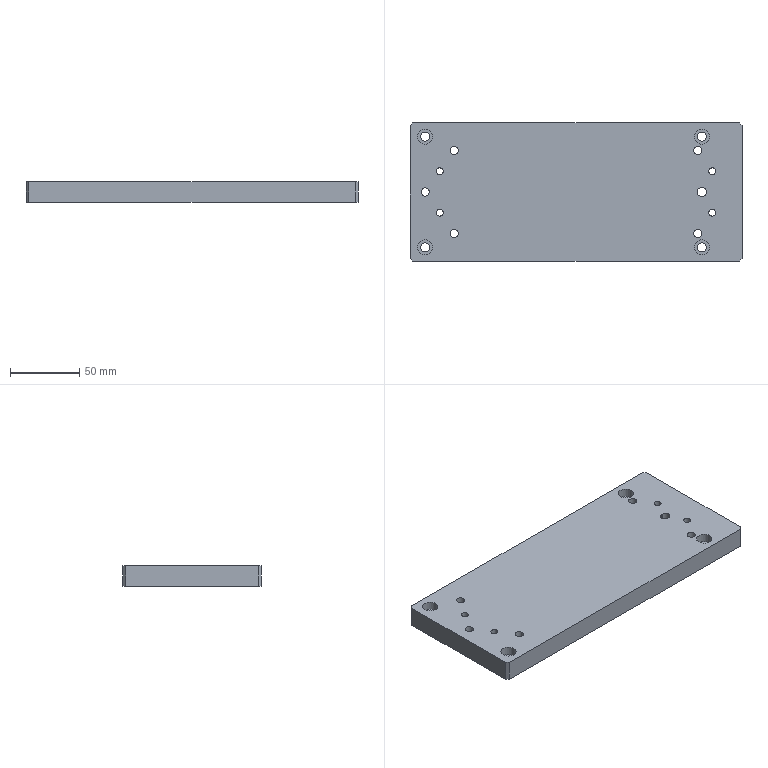Part | NX | 1 solid | 35 faces | box 240 x 100 x 15 mm | volume 352457 mm3 | cylinder 19 | plane 16 | commonest cylinder face diameters 6 x7 5 x4 6.6 x4 11 x4
STEP:
#1=CARTESIAN_POINT('',(-118.,50.,15.));
#2=VERTEX_POINT('',#1);
#3=CARTESIAN_POINT('',(-120.,48.,15.));
#4=VERTEX_POINT('',#3);
#5=CARTESIAN_POINT('',(-84.,84.,15.));
#6=DIRECTION('',(-0.7071,-0.7071,0.));
#7=VECTOR('',#6,1000.);
#8=LINE('',#5,#7);
#9=EDGE_CURVE('',#2,#4,#8,.T.);
#10=ORIENTED_EDGE('',*,*,#9,.F.);
#11=CARTESIAN_POINT('',(-118.,50.,0.));
#12=VERTEX_POINT('',#11);
#13=CARTESIAN_POINT('',(-118.,50.,15.));
#14=DIRECTION('',(0.,0.,1.));
#15=VECTOR('',#14,1000.);
#16=LINE('',#13,#15);
#17=EDGE_CURVE('',#12,#2,#16,.T.);
#18=ORIENTED_EDGE('',*,*,#17,.F.);
#19=CARTESIAN_POINT('',(-120.,48.,0.));
#20=VERTEX_POINT('',#19);
#21=CARTESIAN_POINT('',(-120.,48.,0.));
#22=DIRECTION('',(0.7071,0.7071,0.));
#23=VECTOR('',#22,1000.);
#24=LINE('',#21,#23);
#25=EDGE_CURVE('',#20,#12,#24,.T.);
#26=ORIENTED_EDGE('',*,*,#25,.F.);
#27=CARTESIAN_POINT('',(-120.,48.,15.));
#28=DIRECTION('',(0.,0.,-1.));
#29=VECTOR('',#28,1000.);
#30=LINE('',#27,#29);
#31=EDGE_CURVE('',#4,#20,#30,.T.);
#32=ORIENTED_EDGE('',*,*,#31,.F.);
#33=EDGE_LOOP('',(#10,#18,#26,#32));
#34=FACE_BOUND('',#33,.T.);
#35=CARTESIAN_POINT('',(-120.,48.,15.));
#36=DIRECTION('',(0.7071,-0.7071,0.));
#37=DIRECTION('',(0.,0.,-1.));
#38=AXIS2_PLACEMENT_3D('',#35,#36,#37);
#39=PLANE('',#38);
#40=ADVANCED_FACE('',(#34),#39,.F.);
#41=CARTESIAN_POINT('',(-120.,-48.,15.));
#42=VERTEX_POINT('',#41);
#43=CARTESIAN_POINT('',(-118.,-50.,15.));
#44=VERTEX_POINT('',#43);
#45=CARTESIAN_POINT('',(-84.,-84.,15.));
#46=DIRECTION('',(0.7071,-0.7071,0.));
#47=VECTOR('',#46,1000.);
#48=LINE('',#45,#47);
#49=EDGE_CURVE('',#42,#44,#48,.T.);
#50=ORIENTED_EDGE('',*,*,#49,.F.);
#51=CARTESIAN_POINT('',(-120.,-48.,0.));
#52=VERTEX_POINT('',#51);
#53=CARTESIAN_POINT('',(-120.,-48.,15.));
#54=DIRECTION('',(0.,0.,1.));
#55=VECTOR('',#54,1000.);
#56=LINE('',#53,#55);
#57=EDGE_CURVE('',#52,#42,#56,.T.);
#58=ORIENTED_EDGE('',*,*,#57,.F.);
#59=CARTESIAN_POINT('',(-118.,-50.,0.));
#60=VERTEX_POINT('',#59);
#61=CARTESIAN_POINT('',(-118.,-50.,0.));
#62=DIRECTION('',(-0.7071,0.7071,0.));
#63=VECTOR('',#62,1000.);
#64=LINE('',#61,#63);
#65=EDGE_CURVE('',#60,#52,#64,.T.);
#66=ORIENTED_EDGE('',*,*,#65,.F.);
#67=CARTESIAN_POINT('',(-118.,-50.,15.));
#68=DIRECTION('',(0.,0.,-1.));
#69=VECTOR('',#68,1000.);
#70=LINE('',#67,#69);
#71=EDGE_CURVE('',#44,#60,#70,.T.);
#72=ORIENTED_EDGE('',*,*,#71,.F.);
#73=EDGE_LOOP('',(#50,#58,#66,#72));
#74=FACE_BOUND('',#73,.T.);
#75=CARTESIAN_POINT('',(-118.,-50.,15.));
#76=DIRECTION('',(0.7071,0.7071,0.));
#77=DIRECTION('',(0.,0.,-1.));
#78=AXIS2_PLACEMENT_3D('',#75,#76,#77);
#79=PLANE('',#78);
#80=ADVANCED_FACE('',(#74),#79,.F.);
#81=CARTESIAN_POINT('',(118.,-50.,15.));
#82=VERTEX_POINT('',#81);
#83=CARTESIAN_POINT('',(120.,-48.,15.));
#84=VERTEX_POINT('',#83);
#85=CARTESIAN_POINT('',(84.,-84.,15.));
#86=DIRECTION('',(0.7071,0.7071,0.));
#87=VECTOR('',#86,1000.);
#88=LINE('',#85,#87);
#89=EDGE_CURVE('',#82,#84,#88,.T.);
#90=ORIENTED_EDGE('',*,*,#89,.F.);
#91=CARTESIAN_POINT('',(118.,-50.,0.));
#92=VERTEX_POINT('',#91);
#93=CARTESIAN_POINT('',(118.,-50.,15.));
#94=DIRECTION('',(0.,0.,1.));
#95=VECTOR('',#94,1000.);
#96=LINE('',#93,#95);
#97=EDGE_CURVE('',#92,#82,#96,.T.);
#98=ORIENTED_EDGE('',*,*,#97,.F.);
#99=CARTESIAN_POINT('',(120.,-48.,0.));
#100=VERTEX_POINT('',#99);
#101=CARTESIAN_POINT('',(120.,-48.,0.));
#102=DIRECTION('',(-0.7071,-0.7071,0.));
#103=VECTOR('',#102,1000.);
#104=LINE('',#101,#103);
#105=EDGE_CURVE('',#100,#92,#104,.T.);
#106=ORIENTED_EDGE('',*,*,#105,.F.);
#107=CARTESIAN_POINT('',(120.,-48.,15.));
#108=DIRECTION('',(0.,0.,-1.));
#109=VECTOR('',#108,1000.);
#110=LINE('',#107,#109);
#111=EDGE_CURVE('',#84,#100,#110,.T.);
#112=ORIENTED_EDGE('',*,*,#111,.F.);
#113=EDGE_LOOP('',(#90,#98,#106,#112));
#114=FACE_BOUND('',#113,.T.);
#115=CARTESIAN_POINT('',(120.,-48.,15.));
#116=DIRECTION('',(-0.7071,0.7071,0.));
#117=DIRECTION('',(0.,0.,-1.));
#118=AXIS2_PLACEMENT_3D('',#115,#116,#117);
#119=PLANE('',#118);
#120=ADVANCED_FACE('',(#114),#119,.F.);
#121=CARTESIAN_POINT('',(120.,48.,15.));
#122=VERTEX_POINT('',#121);
#123=CARTESIAN_POINT('',(118.,50.,15.));
#124=VERTEX_POINT('',#123);
#125=CARTESIAN_POINT('',(84.,84.,15.));
#126=DIRECTION('',(-0.7071,0.7071,0.));
#127=VECTOR('',#126,1000.);
#128=LINE('',#125,#127);
#129=EDGE_CURVE('',#122,#124,#128,.T.);
#130=ORIENTED_EDGE('',*,*,#129,.F.);
#131=CARTESIAN_POINT('',(120.,48.,0.));
#132=VERTEX_POINT('',#131);
#133=CARTESIAN_POINT('',(120.,48.,15.));
#134=DIRECTION('',(0.,0.,1.));
#135=VECTOR('',#134,1000.);
#136=LINE('',#133,#135);
#137=EDGE_CURVE('',#132,#122,#136,.T.);
#138=ORIENTED_EDGE('',*,*,#137,.F.);
#139=CARTESIAN_POINT('',(118.,50.,0.));
#140=VERTEX_POINT('',#139);
#141=CARTESIAN_POINT('',(118.,50.,0.));
#142=DIRECTION('',(0.7071,-0.7071,0.));
#143=VECTOR('',#142,1000.);
#144=LINE('',#141,#143);
#145=EDGE_CURVE('',#140,#132,#144,.T.);
#146=ORIENTED_EDGE('',*,*,#145,.F.);
#147=CARTESIAN_POINT('',(118.,50.,15.));
#148=DIRECTION('',(0.,0.,-1.));
#149=VECTOR('',#148,1000.);
#150=LINE('',#147,#149);
#151=EDGE_CURVE('',#124,#140,#150,.T.);
#152=ORIENTED_EDGE('',*,*,#151,.F.);
#153=EDGE_LOOP('',(#130,#138,#146,#152));
#154=FACE_BOUND('',#153,.T.);
#155=CARTESIAN_POINT('',(118.,50.,15.));
#156=DIRECTION('',(-0.7071,-0.7071,0.));
#157=DIRECTION('',(0.,0.,-1.));
#158=AXIS2_PLACEMENT_3D('',#155,#156,#157);
#159=PLANE('',#158);
#160=ADVANCED_FACE('',(#154),#159,.F.);
#161=CARTESIAN_POINT('',(91.5,-3.,15.));
#162=VERTEX_POINT('',#161);
#163=CARTESIAN_POINT('',(91.5,-3.,0.));
#164=VERTEX_POINT('',#163);
#165=CARTESIAN_POINT('',(91.5,-3.,15.));
#166=DIRECTION('',(0.,0.,-1.));
#167=VECTOR('',#166,1000.);
#168=LINE('',#165,#167);
#169=EDGE_CURVE('',#162,#164,#168,.T.);
#170=ORIENTED_EDGE('',*,*,#169,.T.);
#171=CARTESIAN_POINT('',(90.5,-3.,0.));
#172=VERTEX_POINT('',#171);
#173=CARTESIAN_POINT('',(90.5,-3.,0.));
#174=DIRECTION('',(1.,0.,0.));
#175=VECTOR('',#174,1000.);
#176=LINE('',#173,#175);
#177=EDGE_CURVE('',#172,#164,#176,.T.);
#178=ORIENTED_EDGE('',*,*,#177,.F.);
#179=CARTESIAN_POINT('',(90.5,-3.,15.));
#180=VERTEX_POINT('',#179);
#181=CARTESIAN_POINT('',(90.5,-3.,15.));
#182=DIRECTION('',(0.,0.,1.));
#183=VECTOR('',#182,1000.);
#184=LINE('',#181,#183);
#185=EDGE_CURVE('',#172,#180,#184,.T.);
#186=ORIENTED_EDGE('',*,*,#185,.T.);
#187=CARTESIAN_POINT('',(90.5,-3.,15.));
#188=DIRECTION('',(1.,0.,0.));
#189=VECTOR('',#188,1000.);
#190=LINE('',#187,#189);
#191=EDGE_CURVE('',#180,#162,#190,.T.);
#192=ORIENTED_EDGE('',*,*,#191,.T.);
#193=EDGE_LOOP('',(#170,#178,#186,#192));
#194=FACE_BOUND('',#193,.T.);
#195=CARTESIAN_POINT('',(90.5,-3.,15.));
#196=DIRECTION('',(0.,-1.,0.));
#197=DIRECTION('',(1.,0.,0.));
#198=AXIS2_PLACEMENT_3D('',#195,#196,#197);
#199=PLANE('',#198);
#200=ADVANCED_FACE('',(#194),#199,.F.);
#201=CARTESIAN_POINT('',(91.5,3.,0.));
#202=VERTEX_POINT('',#201);
#203=CARTESIAN_POINT('',(91.5,3.,15.));
#204=VERTEX_POINT('',#203);
#205=CARTESIAN_POINT('',(91.5,3.,15.));
#206=DIRECTION('',(0.,0.,1.));
#207=VECTOR('',#206,1000.);
#208=LINE('',#205,#207);
#209=EDGE_CURVE('',#202,#204,#208,.T.);
#210=ORIENTED_EDGE('',*,*,#209,.T.);
#211=CARTESIAN_POINT('',(90.5,3.,15.));
#212=VERTEX_POINT('',#211);
#213=CARTESIAN_POINT('',(90.5,3.,15.));
#214=DIRECTION('',(1.,0.,0.));
#215=VECTOR('',#214,1000.);
#216=LINE('',#213,#215);
#217=EDGE_CURVE('',#212,#204,#216,.T.);
#218=ORIENTED_EDGE('',*,*,#217,.F.);
#219=CARTESIAN_POINT('',(90.5,3.,0.));
#220=VERTEX_POINT('',#219);
#221=CARTESIAN_POINT('',(90.5,3.,15.));
#222=DIRECTION('',(0.,0.,-1.));
#223=VECTOR('',#222,1000.);
#224=LINE('',#221,#223);
#225=EDGE_CURVE('',#212,#220,#224,.T.);
#226=ORIENTED_EDGE('',*,*,#225,.T.);
#227=CARTESIAN_POINT('',(90.5,3.,0.));
#228=DIRECTION('',(1.,0.,0.));
#229=VECTOR('',#228,1000.);
#230=LINE('',#227,#229);
#231=EDGE_CURVE('',#220,#202,#230,.T.);
#232=ORIENTED_EDGE('',*,*,#231,.T.);
#233=EDGE_LOOP('',(#210,#218,#226,#232));
#234=FACE_BOUND('',#233,.T.);
#235=CARTESIAN_POINT('',(90.5,3.,15.));
#236=DIRECTION('',(0.,1.,0.));
#237=DIRECTION('',(-1.,0.,0.));
#238=AXIS2_PLACEMENT_3D('',#235,#236,#237);
#239=PLANE('',#238);
#240=ADVANCED_FACE('',(#234),#239,.F.);
#241=CARTESIAN_POINT('',(90.5,0.,15.));
#242=DIRECTION('',(0.,0.,1.));
#243=DIRECTION('',(1.,0.,0.));
#244=AXIS2_PLACEMENT_3D('',#241,#242,#243);
#245=CIRCLE('',#244,3.);
#246=EDGE_CURVE('',#212,#180,#245,.T.);
#247=ORIENTED_EDGE('',*,*,#246,.T.);
#248=ORIENTED_EDGE('',*,*,#185,.F.);
#249=CARTESIAN_POINT('',(90.5,0.,0.));
#250=DIRECTION('',(0.,0.,1.));
#251=DIRECTION('',(1.,0.,0.));
#252=AXIS2_PLACEMENT_3D('',#249,#250,#251);
#253=CIRCLE('',#252,3.);
#254=EDGE_CURVE('',#220,#172,#253,.T.);
#255=ORIENTED_EDGE('',*,*,#254,.F.);
#256=ORIENTED_EDGE('',*,*,#225,.F.);
#257=EDGE_LOOP('',(#247,#248,#255,#256));
#258=FACE_BOUND('',#257,.T.);
#259=CARTESIAN_POINT('',(90.5,0.,15.));
#260=DIRECTION('',(0.,0.,1.));
#261=DIRECTION('',(1.,0.,0.));
#262=AXIS2_PLACEMENT_3D('',#259,#260,#261);
#263=CYLINDRICAL_SURFACE('',#262,3.);
#264=ADVANCED_FACE('',(#258),#263,.F.);
#265=CARTESIAN_POINT('',(-103.5,-40.,8.6));
#266=VERTEX_POINT('',#265);
#267=CARTESIAN_POINT('',(-109.,-40.,8.6));
#268=DIRECTION('',(0.,0.,1.));
#269=DIRECTION('',(1.,0.,0.));
#270=AXIS2_PLACEMENT_3D('',#267,#268,#269);
#271=CIRCLE('',#270,5.5);
#272=EDGE_CURVE('',#266,#266,#271,.T.);
#273=ORIENTED_EDGE('',*,*,#272,.T.);
#274=EDGE_LOOP('',(#273));
#275=FACE_BOUND('',#274,.T.);
#276=CARTESIAN_POINT('',(-105.7,-40.,8.6));
#277=VERTEX_POINT('',#276);
#278=CARTESIAN_POINT('',(-109.,-40.,8.6));
#279=DIRECTION('',(0.,0.,1.));
#280=DIRECTION('',(1.,0.,0.));
#281=AXIS2_PLACEMENT_3D('',#278,#279,#280);
#282=CIRCLE('',#281,3.3);
#283=EDGE_CURVE('',#277,#277,#282,.T.);
#284=ORIENTED_EDGE('',*,*,#283,.F.);
#285=EDGE_LOOP('',(#284));
#286=FACE_BOUND('',#285,.T.);
#287=CARTESIAN_POINT('',(-105.7,-40.,8.6));
#288=DIRECTION('',(0.,0.,-1.));
#289=DIRECTION('',(-1.,0.,0.));
#290=AXIS2_PLACEMENT_3D('',#287,#288,#289);
#291=PLANE('',#290);
#292=ADVANCED_FACE('',(#275,#286),#291,.F.);
#293=CARTESIAN_POINT('',(-114.5,40.,8.6));
#294=VERTEX_POINT('',#293);
#295=CARTESIAN_POINT('',(-109.,40.,8.6));
#296=DIRECTION('',(0.,0.,1.));
#297=DIRECTION('',(-1.,0.,0.));
#298=AXIS2_PLACEMENT_3D('',#295,#296,#297);
#299=CIRCLE('',#298,5.5);
#300=EDGE_CURVE('',#294,#294,#299,.T.);
#301=ORIENTED_EDGE('',*,*,#300,.T.);
#302=EDGE_LOOP('',(#301));
#303=FACE_BOUND('',#302,.T.);
#304=CARTESIAN_POINT('',(-112.3,40.,8.6));
#305=VERTEX_POINT('',#304);
#306=CARTESIAN_POINT('',(-109.,40.,8.6));
#307=DIRECTION('',(0.,0.,1.));
#308=DIRECTION('',(-1.,0.,0.));
#309=AXIS2_PLACEMENT_3D('',#306,#307,#308);
#310=CIRCLE('',#309,3.3);
#311=EDGE_CURVE('',#305,#305,#310,.T.);
#312=ORIENTED_EDGE('',*,*,#311,.F.);
#313=EDGE_LOOP('',(#312));
#314=FACE_BOUND('',#313,.T.);
#315=CARTESIAN_POINT('',(-105.7,-40.,8.6));
#316=DIRECTION('',(0.,0.,-1.));
#317=DIRECTION('',(-1.,0.,0.));
#318=AXIS2_PLACEMENT_3D('',#315,#316,#317);
#319=PLANE('',#318);
#320=ADVANCED_FACE('',(#303,#314),#319,.F.);
#321=CARTESIAN_POINT('',(85.5,-40.,8.6));
#322=VERTEX_POINT('',#321);
#323=CARTESIAN_POINT('',(91.,-40.,8.6));
#324=DIRECTION('',(0.,0.,1.));
#325=DIRECTION('',(-1.,0.,0.));
#326=AXIS2_PLACEMENT_3D('',#323,#324,#325);
#327=CIRCLE('',#326,5.5);
#328=EDGE_CURVE('',#322,#322,#327,.T.);
#329=ORIENTED_EDGE('',*,*,#328,.T.);
#330=EDGE_LOOP('',(#329));
#331=FACE_BOUND('',#330,.T.);
#332=CARTESIAN_POINT('',(87.7,-40.,8.6));
#333=VERTEX_POINT('',#332);
#334=CARTESIAN_POINT('',(91.,-40.,8.6));
#335=DIRECTION('',(0.,0.,1.));
#336=DIRECTION('',(-1.,0.,0.));
#337=AXIS2_PLACEMENT_3D('',#334,#335,#336);
#338=CIRCLE('',#337,3.3);
#339=EDGE_CURVE('',#333,#333,#338,.T.);
#340=ORIENTED_EDGE('',*,*,#339,.F.);
#341=EDGE_LOOP('',(#340));
#342=FACE_BOUND('',#341,.T.);
#343=CARTESIAN_POINT('',(-105.7,-40.,8.6));
#344=DIRECTION('',(0.,0.,-1.));
#345=DIRECTION('',(-1.,0.,0.));
#346=AXIS2_PLACEMENT_3D('',#343,#344,#345);
#347=PLANE('',#346);
#348=ADVANCED_FACE('',(#331,#342),#347,.F.);
#349=CARTESIAN_POINT('',(85.5,40.,8.6));
#350=VERTEX_POINT('',#349);
#351=CARTESIAN_POINT('',(91.,40.,8.6));
#352=DIRECTION('',(0.,0.,1.));
#353=DIRECTION('',(-1.,0.,0.));
#354=AXIS2_PLACEMENT_3D('',#351,#352,#353);
#355=CIRCLE('',#354,5.5);
#356=EDGE_CURVE('',#350,#350,#355,.T.);
#357=ORIENTED_EDGE('',*,*,#356,.T.);
#358=EDGE_LOOP('',(#357));
#359=FACE_BOUND('',#358,.T.);
#360=CARTESIAN_POINT('',(87.7,40.,8.6));
#361=VERTEX_POINT('',#360);
#362=CARTESIAN_POINT('',(91.,40.,8.6));
#363=DIRECTION('',(0.,0.,1.));
#364=DIRECTION('',(-1.,0.,0.));
#365=AXIS2_PLACEMENT_3D('',#362,#363,#364);
#366=CIRCLE('',#365,3.3);
#367=EDGE_CURVE('',#361,#361,#366,.T.);
#368=ORIENTED_EDGE('',*,*,#367,.F.);
#369=EDGE_LOOP('',(#368));
#370=FACE_BOUND('',#369,.T.);
#371=CARTESIAN_POINT('',(-105.7,-40.,8.6));
#372=DIRECTION('',(0.,0.,-1.));
#373=DIRECTION('',(-1.,0.,0.));
#374=AXIS2_PLACEMENT_3D('',#371,#372,#373);
#375=PLANE('',#374);
#376=ADVANCED_FACE('',(#359,#370),#375,.F.);
#377=CARTESIAN_POINT('',(-120.,50.,0.));
#378=DIRECTION('',(-1.,0.,0.));
#379=VECTOR('',#378,1000.);
#380=LINE('',#377,#379);
#381=EDGE_CURVE('',#140,#12,#380,.T.);
#382=ORIENTED_EDGE('',*,*,#381,.F.);
#383=ORIENTED_EDGE('',*,*,#145,.T.);
#384=CARTESIAN_POINT('',(120.,50.,0.));
#385=DIRECTION('',(0.,1.,0.));
#386=VECTOR('',#385,1000.);
#387=LINE('',#384,#386);
#388=EDGE_CURVE('',#100,#132,#387,.T.);
#389=ORIENTED_EDGE('',*,*,#388,.F.);
#390=ORIENTED_EDGE('',*,*,#105,.T.);
#391=CARTESIAN_POINT('',(-120.,-50.,0.));
#392=DIRECTION('',(1.,0.,0.));
#393=VECTOR('',#392,1000.);
#394=LINE('',#391,#393);
#395=EDGE_CURVE('',#60,#92,#394,.T.);
#396=ORIENTED_EDGE('',*,*,#395,.F.);
#397=ORIENTED_EDGE('',*,*,#65,.T.);
#398=CARTESIAN_POINT('',(-120.,50.,0.));
#399=DIRECTION('',(0.,-1.,0.));
#400=VECTOR('',#399,1000.);
#401=LINE('',#398,#400);
#402=EDGE_CURVE('',#20,#52,#401,.T.);
#403=ORIENTED_EDGE('',*,*,#402,.F.);
#404=ORIENTED_EDGE('',*,*,#25,.T.);
#405=EDGE_LOOP('',(#382,#383,#389,#390,#396,#397,#403,#404));
#406=FACE_BOUND('',#405,.T.);
#407=CARTESIAN_POINT('',(101.,15.,0.));
#408=VERTEX_POINT('',#407);
#409=CARTESIAN_POINT('',(98.5,15.,0.));
#410=DIRECTION('',(0.,0.,1.));
#411=DIRECTION('',(1.,0.,0.));
#412=AXIS2_PLACEMENT_3D('',#409,#410,#411);
#413=CIRCLE('',#412,2.5);
#414=EDGE_CURVE('',#408,#408,#413,.T.);
#415=ORIENTED_EDGE('',*,*,#414,.T.);
#416=EDGE_LOOP('',(#415));
#417=FACE_BOUND('',#416,.T.);
#418=CARTESIAN_POINT('',(101.,-15.,0.));
#419=VERTEX_POINT('',#418);
#420=CARTESIAN_POINT('',(98.5,-15.,0.));
#421=DIRECTION('',(0.,0.,1.));
#422=DIRECTION('',(1.,0.,0.));
#423=AXIS2_PLACEMENT_3D('',#420,#421,#422);
#424=CIRCLE('',#423,2.5);
#425=EDGE_CURVE('',#419,#419,#424,.T.);
#426=ORIENTED_EDGE('',*,*,#425,.T.);
#427=EDGE_LOOP('',(#426));
#428=FACE_BOUND('',#427,.T.);
#429=CARTESIAN_POINT('',(-96.,-15.,0.));
#430=VERTEX_POINT('',#429);
#431=CARTESIAN_POINT('',(-98.5,-15.,0.));
#432=DIRECTION('',(0.,0.,1.));
#433=DIRECTION('',(1.,0.,0.));
#434=AXIS2_PLACEMENT_3D('',#431,#432,#433);
#435=CIRCLE('',#434,2.5);
#436=EDGE_CURVE('',#430,#430,#435,.T.);
#437=ORIENTED_EDGE('',*,*,#436,.T.);
#438=EDGE_LOOP('',(#437));
#439=FACE_BOUND('',#438,.T.);
#440=CARTESIAN_POINT('',(-96.,15.,0.));
#441=VERTEX_POINT('',#440);
#442=CARTESIAN_POINT('',(-98.5,15.,0.));
#443=DIRECTION('',(0.,0.,1.));
#444=DIRECTION('',(1.,0.,0.));
#445=AXIS2_PLACEMENT_3D('',#442,#443,#444);
#446=CIRCLE('',#445,2.5);
#447=EDGE_CURVE('',#441,#441,#446,.T.);
#448=ORIENTED_EDGE('',*,*,#447,.T.);
#449=EDGE_LOOP('',(#448));
#450=FACE_BOUND('',#449,.T.);
#451=CARTESIAN_POINT('',(94.3,40.,0.));
#452=VERTEX_POINT('',#451);
#453=CARTESIAN_POINT('',(91.,40.,0.));
#454=DIRECTION('',(0.,0.,1.));
#455=DIRECTION('',(1.,0.,0.));
#456=AXIS2_PLACEMENT_3D('',#453,#454,#455);
#457=CIRCLE('',#456,3.3);
#458=EDGE_CURVE('',#452,#452,#457,.T.);
#459=ORIENTED_EDGE('',*,*,#458,.T.);
#460=EDGE_LOOP('',(#459));
#461=FACE_BOUND('',#460,.T.);
#462=CARTESIAN_POINT('',(94.3,-40.,0.));
#463=VERTEX_POINT('',#462);
#464=CARTESIAN_POINT('',(91.,-40.,0.));
#465=DIRECTION('',(0.,0.,1.));
#466=DIRECTION('',(1.,0.,0.));
#467=AXIS2_PLACEMENT_3D('',#464,#465,#466);
#468=CIRCLE('',#467,3.3);
#469=EDGE_CURVE('',#463,#463,#468,.T.);
#470=ORIENTED_EDGE('',*,*,#469,.T.);
#471=EDGE_LOOP('',(#470));
#472=FACE_BOUND('',#471,.T.);
#473=CARTESIAN_POINT('',(-105.7,40.,0.));
#474=VERTEX_POINT('',#473);
#475=CARTESIAN_POINT('',(-109.,40.,0.));
#476=DIRECTION('',(0.,0.,1.));
#477=DIRECTION('',(1.,0.,0.));
#478=AXIS2_PLACEMENT_3D('',#475,#476,#477);
#479=CIRCLE('',#478,3.3);
#480=EDGE_CURVE('',#474,#474,#479,.T.);
#481=ORIENTED_EDGE('',*,*,#480,.T.);
#482=EDGE_LOOP('',(#481));
#483=FACE_BOUND('',#482,.T.);
#484=CARTESIAN_POINT('',(-105.7,-40.,0.));
#485=VERTEX_POINT('',#484);
#486=CARTESIAN_POINT('',(-109.,-40.,0.));
#487=DIRECTION('',(0.,0.,1.));
#488=DIRECTION('',(1.,0.,0.));
#489=AXIS2_PLACEMENT_3D('',#486,#487,#488);
#490=CIRCLE('',#489,3.3);
#491=EDGE_CURVE('',#485,#485,#490,.T.);
#492=ORIENTED_EDGE('',*,*,#491,.T.);
#493=EDGE_LOOP('',(#492));
#494=FACE_BOUND('',#493,.T.);
#495=CARTESIAN_POINT('',(-106.,0.,0.));
#496=VERTEX_POINT('',#495);
#497=CARTESIAN_POINT('',(-109.,0.,0.));
#498=DIRECTION('',(0.,0.,1.));
#499=DIRECTION('',(1.,0.,0.));
#500=AXIS2_PLACEMENT_3D('',#497,#498,#499);
#501=CIRCLE('',#500,3.);
#502=EDGE_CURVE('',#496,#496,#501,.T.);
#503=ORIENTED_EDGE('',*,*,#502,.T.);
#504=EDGE_LOOP('',(#503));
#505=FACE_BOUND('',#504,.T.);
#506=ORIENTED_EDGE('',*,*,#177,.T.);
#507=CARTESIAN_POINT('',(91.5,0.,0.));
#508=DIRECTION('',(0.,0.,1.));
#509=DIRECTION('',(1.,0.,0.));
#510=AXIS2_PLACEMENT_3D('',#507,#508,#509);
#511=CIRCLE('',#510,3.);
#512=EDGE_CURVE('',#164,#202,#511,.T.);
#513=ORIENTED_EDGE('',*,*,#512,.T.);
#514=ORIENTED_EDGE('',*,*,#231,.F.);
#515=ORIENTED_EDGE('',*,*,#254,.T.);
#516=EDGE_LOOP('',(#506,#513,#514,#515));
#517=FACE_BOUND('',#516,.T.);
#518=CARTESIAN_POINT('',(91.,-30.,0.));
#519=VERTEX_POINT('',#518);
#520=CARTESIAN_POINT('',(88.,-30.,0.));
#521=DIRECTION('',(0.,0.,1.));
#522=DIRECTION('',(1.,0.,0.));
#523=AXIS2_PLACEMENT_3D('',#520,#521,#522);
#524=CIRCLE('',#523,3.);
#525=EDGE_CURVE('',#519,#519,#524,.T.);
#526=ORIENTED_EDGE('',*,*,#525,.T.);
#527=EDGE_LOOP('',(#526));
#528=FACE_BOUND('',#527,.T.);
#529=CARTESIAN_POINT('',(91.,30.,0.));
#530=VERTEX_POINT('',#529);
#531=CARTESIAN_POINT('',(88.,30.,0.));
#532=DIRECTION('',(0.,0.,1.));
#533=DIRECTION('',(1.,0.,0.));
#534=AXIS2_PLACEMENT_3D('',#531,#532,#533);
#535=CIRCLE('',#534,3.);
#536=EDGE_CURVE('',#530,#530,#535,.T.);
#537=ORIENTED_EDGE('',*,*,#536,.T.);
#538=EDGE_LOOP('',(#537));
#539=FACE_BOUND('',#538,.T.);
#540=CARTESIAN_POINT('',(-85.,-30.,0.));
#541=VERTEX_POINT('',#540);
#542=CARTESIAN_POINT('',(-88.,-30.,0.));
#543=DIRECTION('',(0.,0.,1.));
#544=DIRECTION('',(1.,0.,0.));
#545=AXIS2_PLACEMENT_3D('',#542,#543,#544);
#546=CIRCLE('',#545,3.);
#547=EDGE_CURVE('',#541,#541,#546,.T.);
#548=ORIENTED_EDGE('',*,*,#547,.T.);
#549=EDGE_LOOP('',(#548));
#550=FACE_BOUND('',#549,.T.);
#551=CARTESIAN_POINT('',(-85.,30.,0.));
#552=VERTEX_POINT('',#551);
#553=CARTESIAN_POINT('',(-88.,30.,0.));
#554=DIRECTION('',(0.,0.,1.));
#555=DIRECTION('',(1.,0.,0.));
#556=AXIS2_PLACEMENT_3D('',#553,#554,#555);
#557=CIRCLE('',#556,3.);
#558=EDGE_CURVE('',#552,#552,#557,.T.);
#559=ORIENTED_EDGE('',*,*,#558,.T.);
#560=EDGE_LOOP('',(#559));
#561=FACE_BOUND('',#560,.T.);
#562=CARTESIAN_POINT('',(0.,0.,0.));
#563=DIRECTION('',(0.,0.,1.));
#564=DIRECTION('',(1.,0.,0.));
#565=AXIS2_PLACEMENT_3D('',#562,#563,#564);
#566=PLANE('',#565);
#567=ADVANCED_FACE('',(#406,#417,#428,#439,#450,#461,#472,#483,#494,#505,#517,#528,#539,#550,#561),#566,.F.);
#568=ORIENTED_EDGE('',*,*,#395,.T.);
#569=ORIENTED_EDGE('',*,*,#97,.T.);
#570=CARTESIAN_POINT('',(-120.,-50.,15.));
#571=DIRECTION('',(1.,0.,0.));
#572=VECTOR('',#571,1000.);
#573=LINE('',#570,#572);
#574=EDGE_CURVE('',#44,#82,#573,.T.);
#575=ORIENTED_EDGE('',*,*,#574,.F.);
#576=ORIENTED_EDGE('',*,*,#71,.T.);
#577=EDGE_LOOP('',(#568,#569,#575,#576));
#578=FACE_BOUND('',#577,.T.);
#579=CARTESIAN_POINT('',(-120.,-50.,15.));
#580=DIRECTION('',(0.,1.,0.));
#581=DIRECTION('',(0.,0.,1.));
#582=AXIS2_PLACEMENT_3D('',#579,#580,#581);
#583=PLANE('',#582);
#584=ADVANCED_FACE('',(#578),#583,.F.);
#585=ORIENTED_EDGE('',*,*,#402,.T.);
#586=ORIENTED_EDGE('',*,*,#57,.T.);
#587=CARTESIAN_POINT('',(-120.,50.,15.));
#588=DIRECTION('',(0.,-1.,0.));
#589=VECTOR('',#588,1000.);
#590=LINE('',#587,#589);
#591=EDGE_CURVE('',#4,#42,#590,.T.);
#592=ORIENTED_EDGE('',*,*,#591,.F.);
#593=ORIENTED_EDGE('',*,*,#31,.T.);
#594=EDGE_LOOP('',(#585,#586,#592,#593));
#595=FACE_BOUND('',#594,.T.);
#596=CARTESIAN_POINT('',(-120.,50.,15.));
#597=DIRECTION('',(1.,0.,0.));
#598=DIRECTION('',(0.,1.,0.));
#599=AXIS2_PLACEMENT_3D('',#596,#597,#598);
#600=PLANE('',#599);
#601=ADVANCED_FACE('',(#595),#600,.F.);
#602=CARTESIAN_POINT('',(-120.,50.,15.));
#603=DIRECTION('',(-1.,0.,0.));
#604=VECTOR('',#603,1000.);
#605=LINE('',#602,#604);
#606=EDGE_CURVE('',#124,#2,#605,.T.);
#607=ORIENTED_EDGE('',*,*,#606,.F.);
#608=ORIENTED_EDGE('',*,*,#151,.T.);
#609=ORIENTED_EDGE('',*,*,#381,.T.);
#610=ORIENTED_EDGE('',*,*,#17,.T.);
#611=EDGE_LOOP('',(#607,#608,#609,#610));
#612=FACE_BOUND('',#611,.T.);
#613=CARTESIAN_POINT('',(-120.,50.,15.));
#614=DIRECTION('',(0.,-1.,0.));
#615=DIRECTION('',(0.,0.,-1.));
#616=AXIS2_PLACEMENT_3D('',#613,#614,#615);
#617=PLANE('',#616);
#618=ADVANCED_FACE('',(#612),#617,.F.);
#619=ORIENTED_EDGE('',*,*,#388,.T.);
#620=ORIENTED_EDGE('',*,*,#137,.T.);
#621=CARTESIAN_POINT('',(120.,50.,15.));
#622=DIRECTION('',(0.,1.,0.));
#623=VECTOR('',#622,1000.);
#624=LINE('',#621,#623);
#625=EDGE_CURVE('',#84,#122,#624,.T.);
#626=ORIENTED_EDGE('',*,*,#625,.F.);
#627=ORIENTED_EDGE('',*,*,#111,.T.);
#628=EDGE_LOOP('',(#619,#620,#626,#627));
#629=FACE_BOUND('',#628,.T.);
#630=CARTESIAN_POINT('',(120.,50.,15.));
#631=DIRECTION('',(-1.,0.,0.));
#632=DIRECTION('',(0.,0.,1.));
#633=AXIS2_PLACEMENT_3D('',#630,#631,#632);
#634=PLANE('',#633);
#635=ADVANCED_FACE('',(#629),#634,.F.);
#636=ORIENTED_EDGE('',*,*,#246,.F.);
#637=ORIENTED_EDGE('',*,*,#217,.T.);
#638=CARTESIAN_POINT('',(91.5,0.,15.));
#639=DIRECTION('',(0.,0.,1.));
#640=DIRECTION('',(1.,0.,0.));
#641=AXIS2_PLACEMENT_3D('',#638,#639,#640);
#642=CIRCLE('',#641,3.);
#643=EDGE_CURVE('',#162,#204,#642,.T.);
#644=ORIENTED_EDGE('',*,*,#643,.F.);
#645=ORIENTED_EDGE('',*,*,#191,.F.);
#646=EDGE_LOOP('',(#636,#637,#644,#645));
#647=FACE_BOUND('',#646,.T.);
#648=ORIENTED_EDGE('',*,*,#625,.T.);
#649=ORIENTED_EDGE('',*,*,#129,.T.);
#650=ORIENTED_EDGE('',*,*,#606,.T.);
#651=ORIENTED_EDGE('',*,*,#9,.T.);
#652=ORIENTED_EDGE('',*,*,#591,.T.);
#653=ORIENTED_EDGE('',*,*,#49,.T.);
#654=ORIENTED_EDGE('',*,*,#574,.T.);
#655=ORIENTED_EDGE('',*,*,#89,.T.);
#656=EDGE_LOOP('',(#648,#649,#650,#651,#652,#653,#654,#655));
#657=FACE_BOUND('',#656,.T.);
#658=CARTESIAN_POINT('',(101.,15.,15.));
#659=VERTEX_POINT('',#658);
#660=CARTESIAN_POINT('',(98.5,15.,15.));
#661=DIRECTION('',(0.,0.,1.));
#662=DIRECTION('',(1.,0.,0.));
#663=AXIS2_PLACEMENT_3D('',#660,#661,#662);
#664=CIRCLE('',#663,2.5);
#665=EDGE_CURVE('',#659,#659,#664,.T.);
#666=ORIENTED_EDGE('',*,*,#665,.F.);
#667=EDGE_LOOP('',(#666));
#668=FACE_BOUND('',#667,.T.);
#669=CARTESIAN_POINT('',(101.,-15.,15.));
#670=VERTEX_POINT('',#669);
#671=CARTESIAN_POINT('',(98.5,-15.,15.));
#672=DIRECTION('',(0.,0.,1.));
#673=DIRECTION('',(1.,0.,0.));
#674=AXIS2_PLACEMENT_3D('',#671,#672,#673);
#675=CIRCLE('',#674,2.5);
#676=EDGE_CURVE('',#670,#670,#675,.T.);
#677=ORIENTED_EDGE('',*,*,#676,.F.);
#678=EDGE_LOOP('',(#677));
#679=FACE_BOUND('',#678,.T.);
#680=CARTESIAN_POINT('',(-96.,-15.,15.));
#681=VERTEX_POINT('',#680);
#682=CARTESIAN_POINT('',(-98.5,-15.,15.));
#683=DIRECTION('',(0.,0.,1.));
#684=DIRECTION('',(1.,0.,0.));
#685=AXIS2_PLACEMENT_3D('',#682,#683,#684);
#686=CIRCLE('',#685,2.5);
#687=EDGE_CURVE('',#681,#681,#686,.T.);
#688=ORIENTED_EDGE('',*,*,#687,.F.);
#689=EDGE_LOOP('',(#688));
#690=FACE_BOUND('',#689,.T.);
#691=CARTESIAN_POINT('',(-96.,15.,15.));
#692=VERTEX_POINT('',#691);
#693=CARTESIAN_POINT('',(-98.5,15.,15.));
#694=DIRECTION('',(0.,0.,1.));
#695=DIRECTION('',(1.,0.,0.));
#696=AXIS2_PLACEMENT_3D('',#693,#694,#695);
#697=CIRCLE('',#696,2.5);
#698=EDGE_CURVE('',#692,#692,#697,.T.);
#699=ORIENTED_EDGE('',*,*,#698,.F.);
#700=EDGE_LOOP('',(#699));
#701=FACE_BOUND('',#700,.T.);
#702=CARTESIAN_POINT('',(96.5,40.,15.));
#703=VERTEX_POINT('',#702);
#704=CARTESIAN_POINT('',(91.,40.,15.));
#705=DIRECTION('',(0.,0.,1.));
#706=DIRECTION('',(1.,0.,0.));
#707=AXIS2_PLACEMENT_3D('',#704,#705,#706);
#708=CIRCLE('',#707,5.5);
#709=EDGE_CURVE('',#703,#703,#708,.T.);
#710=ORIENTED_EDGE('',*,*,#709,.F.);
#711=EDGE_LOOP('',(#710));
#712=FACE_BOUND('',#711,.T.);
#713=CARTESIAN_POINT('',(96.5,-40.,15.));
#714=VERTEX_POINT('',#713);
#715=CARTESIAN_POINT('',(91.,-40.,15.));
#716=DIRECTION('',(0.,0.,1.));
#717=DIRECTION('',(1.,0.,0.));
#718=AXIS2_PLACEMENT_3D('',#715,#716,#717);
#719=CIRCLE('',#718,5.5);
#720=EDGE_CURVE('',#714,#714,#719,.T.);
#721=ORIENTED_EDGE('',*,*,#720,.F.);
#722=EDGE_LOOP('',(#721));
#723=FACE_BOUND('',#722,.T.);
#724=CARTESIAN_POINT('',(-103.5,40.,15.));
#725=VERTEX_POINT('',#724);
#726=CARTESIAN_POINT('',(-109.,40.,15.));
#727=DIRECTION('',(0.,0.,1.));
#728=DIRECTION('',(1.,0.,0.));
#729=AXIS2_PLACEMENT_3D('',#726,#727,#728);
#730=CIRCLE('',#729,5.5);
#731=EDGE_CURVE('',#725,#725,#730,.T.);
#732=ORIENTED_EDGE('',*,*,#731,.F.);
#733=EDGE_LOOP('',(#732));
#734=FACE_BOUND('',#733,.T.);
#735=CARTESIAN_POINT('',(-103.5,-40.,15.));
#736=VERTEX_POINT('',#735);
#737=CARTESIAN_POINT('',(-109.,-40.,15.));
#738=DIRECTION('',(0.,0.,1.));
#739=DIRECTION('',(1.,0.,0.));
#740=AXIS2_PLACEMENT_3D('',#737,#738,#739);
#741=CIRCLE('',#740,5.5);
#742=EDGE_CURVE('',#736,#736,#741,.T.);
#743=ORIENTED_EDGE('',*,*,#742,.F.);
#744=EDGE_LOOP('',(#743));
#745=FACE_BOUND('',#744,.T.);
#746=CARTESIAN_POINT('',(-106.,0.,15.));
#747=VERTEX_POINT('',#746);
#748=CARTESIAN_POINT('',(-109.,0.,15.));
#749=DIRECTION('',(0.,0.,1.));
#750=DIRECTION('',(1.,0.,0.));
#751=AXIS2_PLACEMENT_3D('',#748,#749,#750);
#752=CIRCLE('',#751,3.);
#753=EDGE_CURVE('',#747,#747,#752,.T.);
#754=ORIENTED_EDGE('',*,*,#753,.F.);
#755=EDGE_LOOP('',(#754));
#756=FACE_BOUND('',#755,.T.);
#757=CARTESIAN_POINT('',(91.,-30.,15.));
#758=VERTEX_POINT('',#757);
#759=CARTESIAN_POINT('',(88.,-30.,15.));
#760=DIRECTION('',(0.,0.,1.));
#761=DIRECTION('',(1.,0.,0.));
#762=AXIS2_PLACEMENT_3D('',#759,#760,#761);
#763=CIRCLE('',#762,3.);
#764=EDGE_CURVE('',#758,#758,#763,.T.);
#765=ORIENTED_EDGE('',*,*,#764,.F.);
#766=EDGE_LOOP('',(#765));
#767=FACE_BOUND('',#766,.T.);
#768=CARTESIAN_POINT('',(91.,30.,15.));
#769=VERTEX_POINT('',#768);
#770=CARTESIAN_POINT('',(88.,30.,15.));
#771=DIRECTION('',(0.,0.,1.));
#772=DIRECTION('',(1.,0.,0.));
#773=AXIS2_PLACEMENT_3D('',#770,#771,#772);
#774=CIRCLE('',#773,3.);
#775=EDGE_CURVE('',#769,#769,#774,.T.);
#776=ORIENTED_EDGE('',*,*,#775,.F.);
#777=EDGE_LOOP('',(#776));
#778=FACE_BOUND('',#777,.T.);
#779=CARTESIAN_POINT('',(-85.,-30.,15.));
#780=VERTEX_POINT('',#779);
#781=CARTESIAN_POINT('',(-88.,-30.,15.));
#782=DIRECTION('',(0.,0.,1.));
#783=DIRECTION('',(1.,0.,0.));
#784=AXIS2_PLACEMENT_3D('',#781,#782,#783);
#785=CIRCLE('',#784,3.);
#786=EDGE_CURVE('',#780,#780,#785,.T.);
#787=ORIENTED_EDGE('',*,*,#786,.F.);
#788=EDGE_LOOP('',(#787));
#789=FACE_BOUND('',#788,.T.);
#790=CARTESIAN_POINT('',(-85.,30.,15.));
#791=VERTEX_POINT('',#790);
#792=CARTESIAN_POINT('',(-88.,30.,15.));
#793=DIRECTION('',(0.,0.,1.));
#794=DIRECTION('',(1.,0.,0.));
#795=AXIS2_PLACEMENT_3D('',#792,#793,#794);
#796=CIRCLE('',#795,3.);
#797=EDGE_CURVE('',#791,#791,#796,.T.);
#798=ORIENTED_EDGE('',*,*,#797,.F.);
#799=EDGE_LOOP('',(#798));
#800=FACE_BOUND('',#799,.T.);
#801=CARTESIAN_POINT('',(0.,0.,15.));
#802=DIRECTION('',(0.,0.,1.));
#803=DIRECTION('',(1.,0.,0.));
#804=AXIS2_PLACEMENT_3D('',#801,#802,#803);
#805=PLANE('',#804);
#806=ADVANCED_FACE('',(#647,#657,#668,#679,#690,#701,#712,#723,#734,#745,#756,#767,#778,#789,#800),#805,.T.);
#807=ORIENTED_EDGE('',*,*,#414,.F.);
#808=EDGE_LOOP('',(#807));
#809=FACE_BOUND('',#808,.T.);
#810=ORIENTED_EDGE('',*,*,#665,.T.);
#811=EDGE_LOOP('',(#810));
#812=FACE_BOUND('',#811,.T.);
#813=CARTESIAN_POINT('',(98.5,15.,15.));
#814=DIRECTION('',(0.,0.,1.));
#815=DIRECTION('',(1.,0.,0.));
#816=AXIS2_PLACEMENT_3D('',#813,#814,#815);
#817=CYLINDRICAL_SURFACE('',#816,2.5);
#818=ADVANCED_FACE('',(#809,#812),#817,.F.);
#819=ORIENTED_EDGE('',*,*,#425,.F.);
#820=EDGE_LOOP('',(#819));
#821=FACE_BOUND('',#820,.T.);
#822=ORIENTED_EDGE('',*,*,#676,.T.);
#823=EDGE_LOOP('',(#822));
#824=FACE_BOUND('',#823,.T.);
#825=CARTESIAN_POINT('',(98.5,-15.,15.));
#826=DIRECTION('',(0.,0.,1.));
#827=DIRECTION('',(1.,0.,0.));
#828=AXIS2_PLACEMENT_3D('',#825,#826,#827);
#829=CYLINDRICAL_SURFACE('',#828,2.5);
#830=ADVANCED_FACE('',(#821,#824),#829,.F.);
#831=ORIENTED_EDGE('',*,*,#436,.F.);
#832=EDGE_LOOP('',(#831));
#833=FACE_BOUND('',#832,.T.);
#834=ORIENTED_EDGE('',*,*,#687,.T.);
#835=EDGE_LOOP('',(#834));
#836=FACE_BOUND('',#835,.T.);
#837=CARTESIAN_POINT('',(-98.5,-15.,15.));
#838=DIRECTION('',(0.,0.,1.));
#839=DIRECTION('',(1.,0.,0.));
#840=AXIS2_PLACEMENT_3D('',#837,#838,#839);
#841=CYLINDRICAL_SURFACE('',#840,2.5);
#842=ADVANCED_FACE('',(#833,#836),#841,.F.);
#843=ORIENTED_EDGE('',*,*,#447,.F.);
#844=EDGE_LOOP('',(#843));
#845=FACE_BOUND('',#844,.T.);
#846=ORIENTED_EDGE('',*,*,#698,.T.);
#847=EDGE_LOOP('',(#846));
#848=FACE_BOUND('',#847,.T.);
#849=CARTESIAN_POINT('',(-98.5,15.,15.));
#850=DIRECTION('',(0.,0.,1.));
#851=DIRECTION('',(1.,0.,0.));
#852=AXIS2_PLACEMENT_3D('',#849,#850,#851);
#853=CYLINDRICAL_SURFACE('',#852,2.5);
#854=ADVANCED_FACE('',(#845,#848),#853,.F.);
#855=ORIENTED_EDGE('',*,*,#458,.F.);
#856=EDGE_LOOP('',(#855));
#857=FACE_BOUND('',#856,.T.);
#858=ORIENTED_EDGE('',*,*,#367,.T.);
#859=EDGE_LOOP('',(#858));
#860=FACE_BOUND('',#859,.T.);
#861=CARTESIAN_POINT('',(91.,40.,15.));
#862=DIRECTION('',(0.,0.,1.));
#863=DIRECTION('',(1.,0.,0.));
#864=AXIS2_PLACEMENT_3D('',#861,#862,#863);
#865=CYLINDRICAL_SURFACE('',#864,3.3);
#866=ADVANCED_FACE('',(#857,#860),#865,.F.);
#867=ORIENTED_EDGE('',*,*,#356,.F.);
#868=EDGE_LOOP('',(#867));
#869=FACE_BOUND('',#868,.T.);
#870=ORIENTED_EDGE('',*,*,#709,.T.);
#871=EDGE_LOOP('',(#870));
#872=FACE_BOUND('',#871,.T.);
#873=CARTESIAN_POINT('',(91.,40.,15.));
#874=DIRECTION('',(0.,0.,1.));
#875=DIRECTION('',(1.,0.,0.));
#876=AXIS2_PLACEMENT_3D('',#873,#874,#875);
#877=CYLINDRICAL_SURFACE('',#876,5.5);
#878=ADVANCED_FACE('',(#869,#872),#877,.F.);
#879=ORIENTED_EDGE('',*,*,#469,.F.);
#880=EDGE_LOOP('',(#879));
#881=FACE_BOUND('',#880,.T.);
#882=ORIENTED_EDGE('',*,*,#339,.T.);
#883=EDGE_LOOP('',(#882));
#884=FACE_BOUND('',#883,.T.);
#885=CARTESIAN_POINT('',(91.,-40.,15.));
#886=DIRECTION('',(0.,0.,1.));
#887=DIRECTION('',(1.,0.,0.));
#888=AXIS2_PLACEMENT_3D('',#885,#886,#887);
#889=CYLINDRICAL_SURFACE('',#888,3.3);
#890=ADVANCED_FACE('',(#881,#884),#889,.F.);
#891=ORIENTED_EDGE('',*,*,#328,.F.);
#892=EDGE_LOOP('',(#891));
#893=FACE_BOUND('',#892,.T.);
#894=ORIENTED_EDGE('',*,*,#720,.T.);
#895=EDGE_LOOP('',(#894));
#896=FACE_BOUND('',#895,.T.);
#897=CARTESIAN_POINT('',(91.,-40.,15.));
#898=DIRECTION('',(0.,0.,1.));
#899=DIRECTION('',(1.,0.,0.));
#900=AXIS2_PLACEMENT_3D('',#897,#898,#899);
#901=CYLINDRICAL_SURFACE('',#900,5.5);
#902=ADVANCED_FACE('',(#893,#896),#901,.F.);
#903=ORIENTED_EDGE('',*,*,#480,.F.);
#904=EDGE_LOOP('',(#903));
#905=FACE_BOUND('',#904,.T.);
#906=ORIENTED_EDGE('',*,*,#311,.T.);
#907=EDGE_LOOP('',(#906));
#908=FACE_BOUND('',#907,.T.);
#909=CARTESIAN_POINT('',(-109.,40.,15.));
#910=DIRECTION('',(0.,0.,1.));
#911=DIRECTION('',(1.,0.,0.));
#912=AXIS2_PLACEMENT_3D('',#909,#910,#911);
#913=CYLINDRICAL_SURFACE('',#912,3.3);
#914=ADVANCED_FACE('',(#905,#908),#913,.F.);
#915=ORIENTED_EDGE('',*,*,#300,.F.);
#916=EDGE_LOOP('',(#915));
#917=FACE_BOUND('',#916,.T.);
#918=ORIENTED_EDGE('',*,*,#731,.T.);
#919=EDGE_LOOP('',(#918));
#920=FACE_BOUND('',#919,.T.);
#921=CARTESIAN_POINT('',(-109.,40.,15.));
#922=DIRECTION('',(0.,0.,1.));
#923=DIRECTION('',(1.,0.,0.));
#924=AXIS2_PLACEMENT_3D('',#921,#922,#923);
#925=CYLINDRICAL_SURFACE('',#924,5.5);
#926=ADVANCED_FACE('',(#917,#920),#925,.F.);
#927=ORIENTED_EDGE('',*,*,#491,.F.);
#928=EDGE_LOOP('',(#927));
#929=FACE_BOUND('',#928,.T.);
#930=ORIENTED_EDGE('',*,*,#283,.T.);
#931=EDGE_LOOP('',(#930));
#932=FACE_BOUND('',#931,.T.);
#933=CARTESIAN_POINT('',(-109.,-40.,15.));
#934=DIRECTION('',(0.,0.,1.));
#935=DIRECTION('',(1.,0.,0.));
#936=AXIS2_PLACEMENT_3D('',#933,#934,#935);
#937=CYLINDRICAL_SURFACE('',#936,3.3);
#938=ADVANCED_FACE('',(#929,#932),#937,.F.);
#939=ORIENTED_EDGE('',*,*,#272,.F.);
#940=EDGE_LOOP('',(#939));
#941=FACE_BOUND('',#940,.T.);
#942=ORIENTED_EDGE('',*,*,#742,.T.);
#943=EDGE_LOOP('',(#942));
#944=FACE_BOUND('',#943,.T.);
#945=CARTESIAN_POINT('',(-109.,-40.,15.));
#946=DIRECTION('',(0.,0.,1.));
#947=DIRECTION('',(1.,0.,0.));
#948=AXIS2_PLACEMENT_3D('',#945,#946,#947);
#949=CYLINDRICAL_SURFACE('',#948,5.5);
#950=ADVANCED_FACE('',(#941,#944),#949,.F.);
#951=ORIENTED_EDGE('',*,*,#502,.F.);
#952=EDGE_LOOP('',(#951));
#953=FACE_BOUND('',#952,.T.);
#954=ORIENTED_EDGE('',*,*,#753,.T.);
#955=EDGE_LOOP('',(#954));
#956=FACE_BOUND('',#955,.T.);
#957=CARTESIAN_POINT('',(-109.,0.,15.));
#958=DIRECTION('',(0.,0.,1.));
#959=DIRECTION('',(1.,0.,0.));
#960=AXIS2_PLACEMENT_3D('',#957,#958,#959);
#961=CYLINDRICAL_SURFACE('',#960,3.);
#962=ADVANCED_FACE('',(#953,#956),#961,.F.);
#963=ORIENTED_EDGE('',*,*,#512,.F.);
#964=ORIENTED_EDGE('',*,*,#169,.F.);
#965=ORIENTED_EDGE('',*,*,#643,.T.);
#966=ORIENTED_EDGE('',*,*,#209,.F.);
#967=EDGE_LOOP('',(#963,#964,#965,#966));
#968=FACE_BOUND('',#967,.T.);
#969=CARTESIAN_POINT('',(91.5,0.,15.));
#970=DIRECTION('',(0.,0.,1.));
#971=DIRECTION('',(1.,0.,0.));
#972=AXIS2_PLACEMENT_3D('',#969,#970,#971);
#973=CYLINDRICAL_SURFACE('',#972,3.);
#974=ADVANCED_FACE('',(#968),#973,.F.);
#975=ORIENTED_EDGE('',*,*,#525,.F.);
#976=EDGE_LOOP('',(#975));
#977=FACE_BOUND('',#976,.T.);
#978=ORIENTED_EDGE('',*,*,#764,.T.);
#979=EDGE_LOOP('',(#978));
#980=FACE_BOUND('',#979,.T.);
#981=CARTESIAN_POINT('',(88.,-30.,15.));
#982=DIRECTION('',(0.,0.,1.));
#983=DIRECTION('',(1.,0.,0.));
#984=AXIS2_PLACEMENT_3D('',#981,#982,#983);
#985=CYLINDRICAL_SURFACE('',#984,3.);
#986=ADVANCED_FACE('',(#977,#980),#985,.F.);
#987=ORIENTED_EDGE('',*,*,#536,.F.);
#988=EDGE_LOOP('',(#987));
#989=FACE_BOUND('',#988,.T.);
#990=ORIENTED_EDGE('',*,*,#775,.T.);
#991=EDGE_LOOP('',(#990));
#992=FACE_BOUND('',#991,.T.);
#993=CARTESIAN_POINT('',(88.,30.,15.));
#994=DIRECTION('',(0.,0.,1.));
#995=DIRECTION('',(1.,0.,0.));
#996=AXIS2_PLACEMENT_3D('',#993,#994,#995);
#997=CYLINDRICAL_SURFACE('',#996,3.);
#998=ADVANCED_FACE('',(#989,#992),#997,.F.);
#999=ORIENTED_EDGE('',*,*,#547,.F.);
#1000=EDGE_LOOP('',(#999));
#1001=FACE_BOUND('',#1000,.T.);
#1002=ORIENTED_EDGE('',*,*,#786,.T.);
#1003=EDGE_LOOP('',(#1002));
#1004=FACE_BOUND('',#1003,.T.);
#1005=CARTESIAN_POINT('',(-88.,-30.,15.));
#1006=DIRECTION('',(0.,0.,1.));
#1007=DIRECTION('',(1.,0.,0.));
#1008=AXIS2_PLACEMENT_3D('',#1005,#1006,#1007);
#1009=CYLINDRICAL_SURFACE('',#1008,3.);
#1010=ADVANCED_FACE('',(#1001,#1004),#1009,.F.);
#1011=ORIENTED_EDGE('',*,*,#558,.F.);
#1012=EDGE_LOOP('',(#1011));
#1013=FACE_BOUND('',#1012,.T.);
#1014=ORIENTED_EDGE('',*,*,#797,.T.);
#1015=EDGE_LOOP('',(#1014));
#1016=FACE_BOUND('',#1015,.T.);
#1017=CARTESIAN_POINT('',(-88.,30.,15.));
#1018=DIRECTION('',(0.,0.,1.));
#1019=DIRECTION('',(1.,0.,0.));
#1020=AXIS2_PLACEMENT_3D('',#1017,#1018,#1019);
#1021=CYLINDRICAL_SURFACE('',#1020,3.);
#1022=ADVANCED_FACE('',(#1013,#1016),#1021,.F.);
#1023=CLOSED_SHELL('',(#40,#80,#120,#160,#200,#240,#264,#292,#320,#348,#376,#567,#584,#601,#618,#635,#806,#818,#830,#842,#854,#866,#878,#890,#902,#914,#926,#938,#950,#962,#974,#986,#998,#1010,#1022));
#1024=MANIFOLD_SOLID_BREP('',#1023);
#1025=(LENGTH_UNIT()NAMED_UNIT(*)SI_UNIT(.MILLI.,.METRE.));
#1026=UNCERTAINTY_MEASURE_WITH_UNIT(LENGTH_MEASURE(0.00001),#1025,'','');
#1027=(NAMED_UNIT(*)PLANE_ANGLE_UNIT()SI_UNIT($,.RADIAN.));
#1028=(NAMED_UNIT(*)SI_UNIT($,.STERADIAN.)SOLID_ANGLE_UNIT());
#1029=(GEOMETRIC_REPRESENTATION_CONTEXT(3)GLOBAL_UNCERTAINTY_ASSIGNED_CONTEXT((#1026))GLOBAL_UNIT_ASSIGNED_CONTEXT((#1025,#1027,#1028))REPRESENTATION_CONTEXT('',''));
#1030=ADVANCED_BREP_SHAPE_REPRESENTATION('',(#1024),#1029);